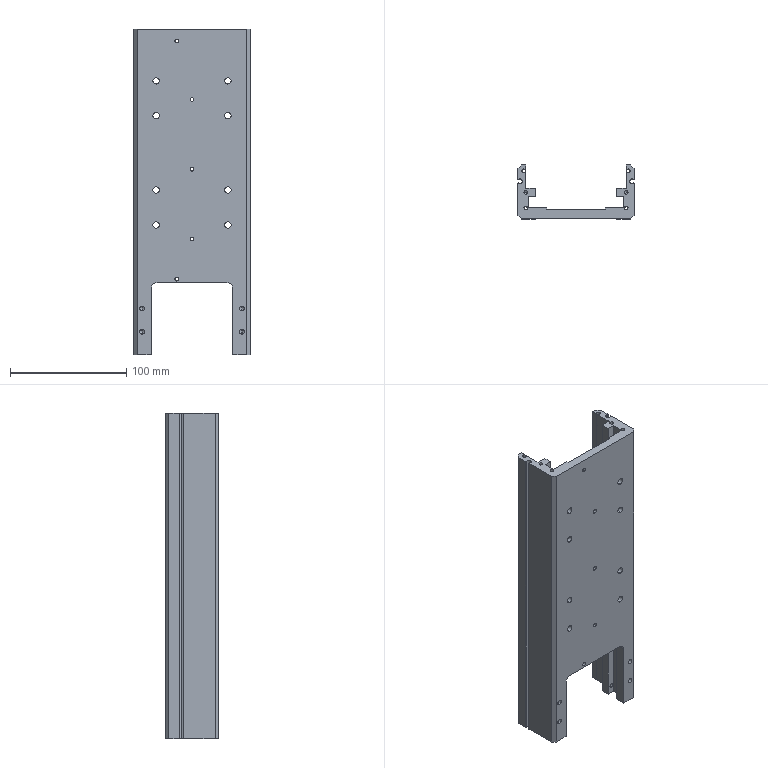Part | SolidWorks | features HoleWzd 7, ICE 5, MirrorPattern 5, 3DProfileFeature 3, Fillet 3, LPattern 3, Cut 2, Chamfer 1, Extrusion 1 | 1 solid | 209 faces | box 100 x 46 x 280 mm | volume 353239 mm3 | cylinder 119 | plane 48 | cone 42 | commonest cylinder face diameters 3.3 x46 11 x24 3.2 x16 5.5 x16 4.2 x8 0.7 x4